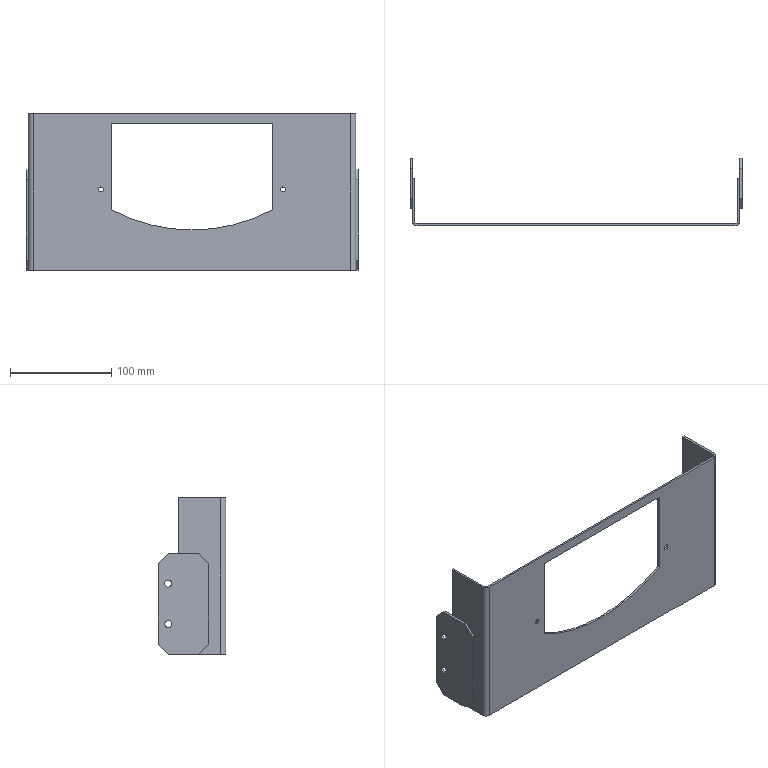Part | NX | features BREP 3 | 3 solids | 50 faces | box 328 x 67 x 155 mm | volume 114572 mm3 | plane 33 | cylinder 17 | commonest cylinder face diameters 7 x8 4.917 x4 6 x2 10 x2 340 x1
STEP:
#1=CARTESIAN_POINT('',(324.,21.928,133.322));
#2=VERTEX_POINT('',#1);
#3=CARTESIAN_POINT('',(326.,21.928,133.322));
#4=VERTEX_POINT('',#3);
#5=CARTESIAN_POINT('',(2.845,21.928,133.322));
#6=DIRECTION('',(-1.,0.,0.));
#7=VECTOR('',#6,1000.);
#8=LINE('',#5,#7);
#9=EDGE_CURVE('',#2,#4,#8,.F.);
#10=ORIENTED_EDGE('',*,*,#9,.T.);
#11=CARTESIAN_POINT('',(326.,28.072,136.678));
#12=VERTEX_POINT('',#11);
#13=CARTESIAN_POINT('',(326.,25.,135.));
#14=DIRECTION('',(-1.,0.,0.));
#15=DIRECTION('',(0.,0.,-1.));
#16=AXIS2_PLACEMENT_3D('',#13,#14,#15);
#17=CIRCLE('',#16,3.5);
#18=EDGE_CURVE('',#12,#4,#17,.T.);
#19=ORIENTED_EDGE('',*,*,#18,.F.);
#20=CARTESIAN_POINT('',(324.,28.072,136.678));
#21=VERTEX_POINT('',#20);
#22=CARTESIAN_POINT('',(2.845,28.072,136.678));
#23=DIRECTION('',(-1.,0.,0.));
#24=VECTOR('',#23,1000.);
#25=LINE('',#22,#24);
#26=EDGE_CURVE('',#21,#12,#25,.F.);
#27=ORIENTED_EDGE('',*,*,#26,.F.);
#28=CARTESIAN_POINT('',(324.,25.,135.));
#29=DIRECTION('',(-1.,0.,0.));
#30=DIRECTION('',(0.,0.,-1.));
#31=AXIS2_PLACEMENT_3D('',#28,#29,#30);
#32=CIRCLE('',#31,3.5);
#33=EDGE_CURVE('',#21,#2,#32,.T.);
#34=ORIENTED_EDGE('',*,*,#33,.T.);
#35=EDGE_LOOP('',(#10,#19,#27,#34));
#36=FACE_BOUND('',#35,.T.);
#37=CARTESIAN_POINT('',(-1.9,25.,135.));
#38=DIRECTION('',(1.,0.,0.));
#39=DIRECTION('',(0.,-0.8776,-0.4794));
#40=AXIS2_PLACEMENT_3D('',#37,#38,#39);
#41=CYLINDRICAL_SURFACE('',#40,3.5);
#42=ADVANCED_FACE('',(#36),#41,.F.);
#43=ORIENTED_EDGE('',*,*,#26,.T.);
#44=CARTESIAN_POINT('',(326.,25.,135.));
#45=DIRECTION('',(-1.,0.,0.));
#46=DIRECTION('',(0.,0.,-1.));
#47=AXIS2_PLACEMENT_3D('',#44,#45,#46);
#48=CIRCLE('',#47,3.5);
#49=EDGE_CURVE('',#4,#12,#48,.T.);
#50=ORIENTED_EDGE('',*,*,#49,.F.);
#51=ORIENTED_EDGE('',*,*,#9,.F.);
#52=CARTESIAN_POINT('',(324.,25.,135.));
#53=DIRECTION('',(-1.,0.,0.));
#54=DIRECTION('',(0.,0.,-1.));
#55=AXIS2_PLACEMENT_3D('',#52,#53,#54);
#56=CIRCLE('',#55,3.5);
#57=EDGE_CURVE('',#2,#21,#56,.T.);
#58=ORIENTED_EDGE('',*,*,#57,.T.);
#59=EDGE_LOOP('',(#43,#50,#51,#58));
#60=FACE_BOUND('',#59,.T.);
#61=CARTESIAN_POINT('',(-1.9,25.,135.));
#62=DIRECTION('',(1.,0.,0.));
#63=DIRECTION('',(0.,-0.8776,-0.4794));
#64=AXIS2_PLACEMENT_3D('',#61,#62,#63);
#65=CYLINDRICAL_SURFACE('',#64,3.5);
#66=ADVANCED_FACE('',(#60),#65,.F.);
#67=CARTESIAN_POINT('',(326.,-15.,115.));
#68=VERTEX_POINT('',#67);
#69=CARTESIAN_POINT('',(326.,-15.,195.));
#70=VERTEX_POINT('',#69);
#71=CARTESIAN_POINT('',(326.,-15.,155.));
#72=DIRECTION('',(0.,0.,1.));
#73=VECTOR('',#72,1000.);
#74=LINE('',#71,#73);
#75=EDGE_CURVE('',#68,#70,#74,.T.);
#76=ORIENTED_EDGE('',*,*,#75,.T.);
#77=CARTESIAN_POINT('',(324.,-15.,195.));
#78=VERTEX_POINT('',#77);
#79=CARTESIAN_POINT('',(325.,-15.,195.));
#80=DIRECTION('',(-1.,0.,0.));
#81=VECTOR('',#80,1000.);
#82=LINE('',#79,#81);
#83=EDGE_CURVE('',#70,#78,#82,.T.);
#84=ORIENTED_EDGE('',*,*,#83,.T.);
#85=CARTESIAN_POINT('',(324.,-15.,115.));
#86=VERTEX_POINT('',#85);
#87=CARTESIAN_POINT('',(324.,-15.,155.));
#88=DIRECTION('',(0.,0.,1.));
#89=VECTOR('',#88,1000.);
#90=LINE('',#87,#89);
#91=EDGE_CURVE('',#86,#78,#90,.T.);
#92=ORIENTED_EDGE('',*,*,#91,.F.);
#93=CARTESIAN_POINT('',(325.,-15.,115.));
#94=DIRECTION('',(-1.,0.,0.));
#95=VECTOR('',#94,1000.);
#96=LINE('',#93,#95);
#97=EDGE_CURVE('',#68,#86,#96,.T.);
#98=ORIENTED_EDGE('',*,*,#97,.F.);
#99=EDGE_LOOP('',(#76,#84,#92,#98));
#100=FACE_BOUND('',#99,.T.);
#101=CARTESIAN_POINT('',(0.,-15.,105.));
#102=DIRECTION('',(0.,-1.,0.));
#103=DIRECTION('',(0.,0.,-1.));
#104=AXIS2_PLACEMENT_3D('',#101,#102,#103);
#105=PLANE('',#104);
#106=ADVANCED_FACE('',(#100),#105,.T.);
#107=CARTESIAN_POINT('',(326.,25.,205.));
#108=VERTEX_POINT('',#107);
#109=CARTESIAN_POINT('',(324.,25.,205.));
#110=VERTEX_POINT('',#109);
#111=CARTESIAN_POINT('',(325.,25.,205.));
#112=DIRECTION('',(-1.,0.,0.));
#113=VECTOR('',#112,1000.);
#114=LINE('',#111,#113);
#115=EDGE_CURVE('',#108,#110,#114,.T.);
#116=ORIENTED_EDGE('',*,*,#115,.T.);
#117=CARTESIAN_POINT('',(324.,-5.,205.));
#118=VERTEX_POINT('',#117);
#119=CARTESIAN_POINT('',(324.,10.,205.));
#120=DIRECTION('',(0.,1.,0.));
#121=VECTOR('',#120,1000.);
#122=LINE('',#119,#121);
#123=EDGE_CURVE('',#118,#110,#122,.T.);
#124=ORIENTED_EDGE('',*,*,#123,.F.);
#125=CARTESIAN_POINT('',(326.,-5.,205.));
#126=VERTEX_POINT('',#125);
#127=CARTESIAN_POINT('',(325.,-5.,205.));
#128=DIRECTION('',(-1.,0.,0.));
#129=VECTOR('',#128,1000.);
#130=LINE('',#127,#129);
#131=EDGE_CURVE('',#126,#118,#130,.T.);
#132=ORIENTED_EDGE('',*,*,#131,.F.);
#133=CARTESIAN_POINT('',(326.,10.,205.));
#134=DIRECTION('',(0.,1.,0.));
#135=VECTOR('',#134,1000.);
#136=LINE('',#133,#135);
#137=EDGE_CURVE('',#126,#108,#136,.T.);
#138=ORIENTED_EDGE('',*,*,#137,.T.);
#139=EDGE_LOOP('',(#116,#124,#132,#138));
#140=FACE_BOUND('',#139,.T.);
#141=CARTESIAN_POINT('',(0.,35.,205.));
#142=DIRECTION('',(0.,0.,-1.));
#143=DIRECTION('',(0.,1.,0.));
#144=AXIS2_PLACEMENT_3D('',#141,#142,#143);
#145=PLANE('',#144);
#146=ADVANCED_FACE('',(#140),#145,.F.);
#147=CARTESIAN_POINT('',(324.,35.,195.));
#148=VERTEX_POINT('',#147);
#149=CARTESIAN_POINT('',(324.,35.,115.));
#150=VERTEX_POINT('',#149);
#151=CARTESIAN_POINT('',(324.,35.,155.));
#152=DIRECTION('',(0.,0.,-1.));
#153=VECTOR('',#152,1000.);
#154=LINE('',#151,#153);
#155=EDGE_CURVE('',#148,#150,#154,.T.);
#156=ORIENTED_EDGE('',*,*,#155,.F.);
#157=CARTESIAN_POINT('',(326.,35.,195.));
#158=VERTEX_POINT('',#157);
#159=CARTESIAN_POINT('',(325.,35.,195.));
#160=DIRECTION('',(-1.,0.,0.));
#161=VECTOR('',#160,1000.);
#162=LINE('',#159,#161);
#163=EDGE_CURVE('',#158,#148,#162,.T.);
#164=ORIENTED_EDGE('',*,*,#163,.F.);
#165=CARTESIAN_POINT('',(326.,35.,115.));
#166=VERTEX_POINT('',#165);
#167=CARTESIAN_POINT('',(326.,35.,155.));
#168=DIRECTION('',(0.,0.,-1.));
#169=VECTOR('',#168,1000.);
#170=LINE('',#167,#169);
#171=EDGE_CURVE('',#158,#166,#170,.T.);
#172=ORIENTED_EDGE('',*,*,#171,.T.);
#173=CARTESIAN_POINT('',(325.,35.,115.));
#174=DIRECTION('',(-1.,0.,0.));
#175=VECTOR('',#174,1000.);
#176=LINE('',#173,#175);
#177=EDGE_CURVE('',#166,#150,#176,.T.);
#178=ORIENTED_EDGE('',*,*,#177,.T.);
#179=EDGE_LOOP('',(#156,#164,#172,#178));
#180=FACE_BOUND('',#179,.T.);
#181=CARTESIAN_POINT('',(0.,35.,205.));
#182=DIRECTION('',(0.,1.,0.));
#183=DIRECTION('',(0.,0.,1.));
#184=AXIS2_PLACEMENT_3D('',#181,#182,#183);
#185=PLANE('',#184);
#186=ADVANCED_FACE('',(#180),#185,.T.);
#187=CARTESIAN_POINT('',(326.,-5.,105.));
#188=VERTEX_POINT('',#187);
#189=CARTESIAN_POINT('',(324.,-5.,105.));
#190=VERTEX_POINT('',#189);
#191=CARTESIAN_POINT('',(325.,-5.,105.));
#192=DIRECTION('',(-1.,0.,0.));
#193=VECTOR('',#192,1000.);
#194=LINE('',#191,#193);
#195=EDGE_CURVE('',#188,#190,#194,.T.);
#196=ORIENTED_EDGE('',*,*,#195,.T.);
#197=CARTESIAN_POINT('',(324.,25.,105.));
#198=VERTEX_POINT('',#197);
#199=CARTESIAN_POINT('',(324.,10.,105.));
#200=DIRECTION('',(0.,-1.,0.));
#201=VECTOR('',#200,1000.);
#202=LINE('',#199,#201);
#203=EDGE_CURVE('',#198,#190,#202,.T.);
#204=ORIENTED_EDGE('',*,*,#203,.F.);
#205=CARTESIAN_POINT('',(326.,25.,105.));
#206=VERTEX_POINT('',#205);
#207=CARTESIAN_POINT('',(325.,25.,105.));
#208=DIRECTION('',(-1.,0.,0.));
#209=VECTOR('',#208,1000.);
#210=LINE('',#207,#209);
#211=EDGE_CURVE('',#206,#198,#210,.T.);
#212=ORIENTED_EDGE('',*,*,#211,.F.);
#213=CARTESIAN_POINT('',(326.,10.,105.));
#214=DIRECTION('',(0.,-1.,0.));
#215=VECTOR('',#214,1000.);
#216=LINE('',#213,#215);
#217=EDGE_CURVE('',#206,#188,#216,.T.);
#218=ORIENTED_EDGE('',*,*,#217,.T.);
#219=EDGE_LOOP('',(#196,#204,#212,#218));
#220=FACE_BOUND('',#219,.T.);
#221=CARTESIAN_POINT('',(0.,-15.,105.));
#222=DIRECTION('',(0.,0.,1.));
#223=DIRECTION('',(0.,-1.,0.));
#224=AXIS2_PLACEMENT_3D('',#221,#222,#223);
#225=PLANE('',#224);
#226=ADVANCED_FACE('',(#220),#225,.F.);
#227=CARTESIAN_POINT('',(324.,-10.,110.));
#228=DIRECTION('',(0.,0.7071,-0.7071));
#229=VECTOR('',#228,1000.);
#230=LINE('',#227,#229);
#231=EDGE_CURVE('',#86,#190,#230,.T.);
#232=ORIENTED_EDGE('',*,*,#231,.T.);
#233=ORIENTED_EDGE('',*,*,#195,.F.);
#234=CARTESIAN_POINT('',(326.,-10.,110.));
#235=DIRECTION('',(0.,-0.7071,0.7071));
#236=VECTOR('',#235,1000.);
#237=LINE('',#234,#236);
#238=EDGE_CURVE('',#188,#68,#237,.T.);
#239=ORIENTED_EDGE('',*,*,#238,.T.);
#240=ORIENTED_EDGE('',*,*,#97,.T.);
#241=EDGE_LOOP('',(#232,#233,#239,#240));
#242=FACE_BOUND('',#241,.T.);
#243=CARTESIAN_POINT('',(-2.4,-5.,105.));
#244=DIRECTION('',(0.,-0.7071,-0.7071));
#245=DIRECTION('',(-1.,0.,0.));
#246=AXIS2_PLACEMENT_3D('',#243,#244,#245);
#247=PLANE('',#246);
#248=ADVANCED_FACE('',(#242),#247,.T.);
#249=CARTESIAN_POINT('',(324.,30.,110.));
#250=DIRECTION('',(0.,0.7071,0.7071));
#251=VECTOR('',#250,1000.);
#252=LINE('',#249,#251);
#253=EDGE_CURVE('',#198,#150,#252,.T.);
#254=ORIENTED_EDGE('',*,*,#253,.T.);
#255=ORIENTED_EDGE('',*,*,#177,.F.);
#256=CARTESIAN_POINT('',(326.,30.,110.));
#257=DIRECTION('',(0.,-0.7071,-0.7071));
#258=VECTOR('',#257,1000.);
#259=LINE('',#256,#258);
#260=EDGE_CURVE('',#166,#206,#259,.T.);
#261=ORIENTED_EDGE('',*,*,#260,.T.);
#262=ORIENTED_EDGE('',*,*,#211,.T.);
#263=EDGE_LOOP('',(#254,#255,#261,#262));
#264=FACE_BOUND('',#263,.T.);
#265=CARTESIAN_POINT('',(0.4,25.,105.));
#266=DIRECTION('',(0.,0.7071,-0.7071));
#267=DIRECTION('',(1.,0.,0.));
#268=AXIS2_PLACEMENT_3D('',#265,#266,#267);
#269=PLANE('',#268);
#270=ADVANCED_FACE('',(#264),#269,.T.);
#271=CARTESIAN_POINT('',(324.,30.,200.));
#272=DIRECTION('',(0.,-0.7071,0.7071));
#273=VECTOR('',#272,1000.);
#274=LINE('',#271,#273);
#275=EDGE_CURVE('',#148,#110,#274,.T.);
#276=ORIENTED_EDGE('',*,*,#275,.T.);
#277=ORIENTED_EDGE('',*,*,#115,.F.);
#278=CARTESIAN_POINT('',(326.,30.,200.));
#279=DIRECTION('',(0.,0.7071,-0.7071));
#280=VECTOR('',#279,1000.);
#281=LINE('',#278,#280);
#282=EDGE_CURVE('',#108,#158,#281,.T.);
#283=ORIENTED_EDGE('',*,*,#282,.T.);
#284=ORIENTED_EDGE('',*,*,#163,.T.);
#285=EDGE_LOOP('',(#276,#277,#283,#284));
#286=FACE_BOUND('',#285,.T.);
#287=CARTESIAN_POINT('',(-2.4,25.,205.));
#288=DIRECTION('',(0.,0.7071,0.7071));
#289=DIRECTION('',(-1.,0.,0.));
#290=AXIS2_PLACEMENT_3D('',#287,#288,#289);
#291=PLANE('',#290);
#292=ADVANCED_FACE('',(#286),#291,.T.);
#293=CARTESIAN_POINT('',(324.,-10.,200.));
#294=DIRECTION('',(0.,-0.7071,-0.7071));
#295=VECTOR('',#294,1000.);
#296=LINE('',#293,#295);
#297=EDGE_CURVE('',#118,#78,#296,.T.);
#298=ORIENTED_EDGE('',*,*,#297,.T.);
#299=ORIENTED_EDGE('',*,*,#83,.F.);
#300=CARTESIAN_POINT('',(326.,-10.,200.));
#301=DIRECTION('',(0.,0.7071,0.7071));
#302=VECTOR('',#301,1000.);
#303=LINE('',#300,#302);
#304=EDGE_CURVE('',#70,#126,#303,.T.);
#305=ORIENTED_EDGE('',*,*,#304,.T.);
#306=ORIENTED_EDGE('',*,*,#131,.T.);
#307=EDGE_LOOP('',(#298,#299,#305,#306));
#308=FACE_BOUND('',#307,.T.);
#309=CARTESIAN_POINT('',(0.4,-5.,205.));
#310=DIRECTION('',(0.,-0.7071,0.7071));
#311=DIRECTION('',(1.,0.,0.));
#312=AXIS2_PLACEMENT_3D('',#309,#310,#311);
#313=PLANE('',#312);
#314=ADVANCED_FACE('',(#308),#313,.T.);
#315=ORIENTED_EDGE('',*,*,#238,.F.);
#316=ORIENTED_EDGE('',*,*,#217,.F.);
#317=ORIENTED_EDGE('',*,*,#260,.F.);
#318=ORIENTED_EDGE('',*,*,#171,.F.);
#319=ORIENTED_EDGE('',*,*,#282,.F.);
#320=ORIENTED_EDGE('',*,*,#137,.F.);
#321=ORIENTED_EDGE('',*,*,#304,.F.);
#322=ORIENTED_EDGE('',*,*,#75,.F.);
#323=EDGE_LOOP('',(#315,#316,#317,#318,#319,#320,#321,#322));
#324=FACE_BOUND('',#323,.T.);
#325=CARTESIAN_POINT('',(326.,21.928,173.322));
#326=VERTEX_POINT('',#325);
#327=CARTESIAN_POINT('',(326.,28.072,176.678));
#328=VERTEX_POINT('',#327);
#329=CARTESIAN_POINT('',(326.,25.,175.));
#330=DIRECTION('',(-1.,0.,0.));
#331=DIRECTION('',(0.,0.,1.));
#332=AXIS2_PLACEMENT_3D('',#329,#330,#331);
#333=CIRCLE('',#332,3.5);
#334=EDGE_CURVE('',#326,#328,#333,.T.);
#335=ORIENTED_EDGE('',*,*,#334,.T.);
#336=CARTESIAN_POINT('',(326.,25.,175.));
#337=DIRECTION('',(-1.,0.,0.));
#338=DIRECTION('',(0.,0.,1.));
#339=AXIS2_PLACEMENT_3D('',#336,#337,#338);
#340=CIRCLE('',#339,3.5);
#341=EDGE_CURVE('',#328,#326,#340,.T.);
#342=ORIENTED_EDGE('',*,*,#341,.T.);
#343=EDGE_LOOP('',(#335,#342));
#344=FACE_BOUND('',#343,.T.);
#345=ORIENTED_EDGE('',*,*,#18,.T.);
#346=ORIENTED_EDGE('',*,*,#49,.T.);
#347=EDGE_LOOP('',(#345,#346));
#348=FACE_BOUND('',#347,.T.);
#349=CARTESIAN_POINT('',(326.,0.,0.));
#350=DIRECTION('',(-1.,0.,0.));
#351=DIRECTION('',(0.,1.,0.));
#352=AXIS2_PLACEMENT_3D('',#349,#350,#351);
#353=PLANE('',#352);
#354=ADVANCED_FACE('',(#324,#344,#348),#353,.F.);
#355=ORIENTED_EDGE('',*,*,#91,.T.);
#356=ORIENTED_EDGE('',*,*,#297,.F.);
#357=ORIENTED_EDGE('',*,*,#123,.T.);
#358=ORIENTED_EDGE('',*,*,#275,.F.);
#359=ORIENTED_EDGE('',*,*,#155,.T.);
#360=ORIENTED_EDGE('',*,*,#253,.F.);
#361=ORIENTED_EDGE('',*,*,#203,.T.);
#362=ORIENTED_EDGE('',*,*,#231,.F.);
#363=EDGE_LOOP('',(#355,#356,#357,#358,#359,#360,#361,#362));
#364=FACE_BOUND('',#363,.T.);
#365=CARTESIAN_POINT('',(324.,28.072,176.678));
#366=VERTEX_POINT('',#365);
#367=CARTESIAN_POINT('',(324.,21.928,173.322));
#368=VERTEX_POINT('',#367);
#369=CARTESIAN_POINT('',(324.,25.,175.));
#370=DIRECTION('',(-1.,0.,0.));
#371=DIRECTION('',(0.,0.,1.));
#372=AXIS2_PLACEMENT_3D('',#369,#370,#371);
#373=CIRCLE('',#372,3.5);
#374=EDGE_CURVE('',#366,#368,#373,.T.);
#375=ORIENTED_EDGE('',*,*,#374,.F.);
#376=CARTESIAN_POINT('',(324.,25.,175.));
#377=DIRECTION('',(-1.,0.,0.));
#378=DIRECTION('',(0.,0.,1.));
#379=AXIS2_PLACEMENT_3D('',#376,#377,#378);
#380=CIRCLE('',#379,3.5);
#381=EDGE_CURVE('',#368,#366,#380,.T.);
#382=ORIENTED_EDGE('',*,*,#381,.F.);
#383=EDGE_LOOP('',(#375,#382));
#384=FACE_BOUND('',#383,.T.);
#385=ORIENTED_EDGE('',*,*,#57,.F.);
#386=ORIENTED_EDGE('',*,*,#33,.F.);
#387=EDGE_LOOP('',(#385,#386));
#388=FACE_BOUND('',#387,.T.);
#389=CARTESIAN_POINT('',(324.,0.,0.));
#390=DIRECTION('',(-1.,0.,0.));
#391=DIRECTION('',(0.,1.,0.));
#392=AXIS2_PLACEMENT_3D('',#389,#390,#391);
#393=PLANE('',#392);
#394=ADVANCED_FACE('',(#364,#384,#388),#393,.T.);
#395=CARTESIAN_POINT('',(2.845,21.928,173.322));
#396=DIRECTION('',(-1.,0.,0.));
#397=VECTOR('',#396,1000.);
#398=LINE('',#395,#397);
#399=EDGE_CURVE('',#368,#326,#398,.F.);
#400=ORIENTED_EDGE('',*,*,#399,.T.);
#401=ORIENTED_EDGE('',*,*,#341,.F.);
#402=CARTESIAN_POINT('',(2.845,28.072,176.678));
#403=DIRECTION('',(-1.,0.,0.));
#404=VECTOR('',#403,1000.);
#405=LINE('',#402,#404);
#406=EDGE_CURVE('',#366,#328,#405,.F.);
#407=ORIENTED_EDGE('',*,*,#406,.F.);
#408=ORIENTED_EDGE('',*,*,#374,.T.);
#409=EDGE_LOOP('',(#400,#401,#407,#408));
#410=FACE_BOUND('',#409,.T.);
#411=CARTESIAN_POINT('',(-1.9,25.,175.));
#412=DIRECTION('',(1.,0.,0.));
#413=DIRECTION('',(0.,-0.8776,-0.4794));
#414=AXIS2_PLACEMENT_3D('',#411,#412,#413);
#415=CYLINDRICAL_SURFACE('',#414,3.5);
#416=ADVANCED_FACE('',(#410),#415,.F.);
#417=ORIENTED_EDGE('',*,*,#406,.T.);
#418=ORIENTED_EDGE('',*,*,#334,.F.);
#419=ORIENTED_EDGE('',*,*,#399,.F.);
#420=ORIENTED_EDGE('',*,*,#381,.T.);
#421=EDGE_LOOP('',(#417,#418,#419,#420));
#422=FACE_BOUND('',#421,.T.);
#423=CARTESIAN_POINT('',(-1.9,25.,175.));
#424=DIRECTION('',(1.,0.,0.));
#425=DIRECTION('',(0.,-0.8776,-0.4794));
#426=AXIS2_PLACEMENT_3D('',#423,#424,#425);
#427=CYLINDRICAL_SURFACE('',#426,3.5);
#428=ADVANCED_FACE('',(#422),#427,.F.);
#429=CLOSED_SHELL('',(#42,#66,#106,#146,#186,#226,#248,#270,#292,#314,#354,#394,#416,#428));
#430=MANIFOLD_SOLID_BREP('',#429);
#431=CARTESIAN_POINT('',(69.842,-32.,186.179));
#432=VERTEX_POINT('',#431);
#433=CARTESIAN_POINT('',(69.842,-30.,186.179));
#434=VERTEX_POINT('',#433);
#435=CARTESIAN_POINT('',(69.842,-27.155,186.179));
#436=DIRECTION('',(0.,-1.,0.));
#437=VECTOR('',#436,1000.);
#438=LINE('',#435,#437);
#439=EDGE_CURVE('',#432,#434,#438,.F.);
#440=ORIENTED_EDGE('',*,*,#439,.T.);
#441=CARTESIAN_POINT('',(74.157,-30.,183.821));
#442=VERTEX_POINT('',#441);
#443=CARTESIAN_POINT('',(72.,-30.,185.));
#444=DIRECTION('',(0.,-1.,0.));
#445=DIRECTION('',(1.,0.,0.));
#446=AXIS2_PLACEMENT_3D('',#443,#444,#445);
#447=CIRCLE('',#446,2.458);
#448=EDGE_CURVE('',#442,#434,#447,.T.);
#449=ORIENTED_EDGE('',*,*,#448,.F.);
#450=CARTESIAN_POINT('',(74.157,-32.,183.821));
#451=VERTEX_POINT('',#450);
#452=CARTESIAN_POINT('',(74.157,-27.155,183.821));
#453=DIRECTION('',(0.,-1.,0.));
#454=VECTOR('',#453,1000.);
#455=LINE('',#452,#454);
#456=EDGE_CURVE('',#451,#442,#455,.F.);
#457=ORIENTED_EDGE('',*,*,#456,.F.);
#458=CARTESIAN_POINT('',(72.,-32.,185.));
#459=DIRECTION('',(0.,-1.,0.));
#460=DIRECTION('',(1.,0.,0.));
#461=AXIS2_PLACEMENT_3D('',#458,#459,#460);
#462=CIRCLE('',#461,2.458);
#463=EDGE_CURVE('',#451,#432,#462,.T.);
#464=ORIENTED_EDGE('',*,*,#463,.T.);
#465=EDGE_LOOP('',(#440,#449,#457,#464));
#466=FACE_BOUND('',#465,.T.);
#467=CARTESIAN_POINT('',(72.,-31.9,185.));
#468=DIRECTION('',(0.,1.,0.));
#469=DIRECTION('',(-0.8776,0.,0.4794));
#470=AXIS2_PLACEMENT_3D('',#467,#468,#469);
#471=CYLINDRICAL_SURFACE('',#470,2.458);
#472=ADVANCED_FACE('',(#466),#471,.F.);
#473=ORIENTED_EDGE('',*,*,#456,.T.);
#474=CARTESIAN_POINT('',(72.,-30.,185.));
#475=DIRECTION('',(0.,-1.,0.));
#476=DIRECTION('',(1.,0.,0.));
#477=AXIS2_PLACEMENT_3D('',#474,#475,#476);
#478=CIRCLE('',#477,2.458);
#479=EDGE_CURVE('',#434,#442,#478,.T.);
#480=ORIENTED_EDGE('',*,*,#479,.F.);
#481=ORIENTED_EDGE('',*,*,#439,.F.);
#482=CARTESIAN_POINT('',(72.,-32.,185.));
#483=DIRECTION('',(0.,-1.,0.));
#484=DIRECTION('',(1.,0.,0.));
#485=AXIS2_PLACEMENT_3D('',#482,#483,#484);
#486=CIRCLE('',#485,2.458);
#487=EDGE_CURVE('',#432,#451,#486,.T.);
#488=ORIENTED_EDGE('',*,*,#487,.T.);
#489=EDGE_LOOP('',(#473,#480,#481,#488));
#490=FACE_BOUND('',#489,.T.);
#491=CARTESIAN_POINT('',(72.,-31.9,185.));
#492=DIRECTION('',(0.,1.,0.));
#493=DIRECTION('',(-0.8776,0.,0.4794));
#494=AXIS2_PLACEMENT_3D('',#491,#492,#493);
#495=CYLINDRICAL_SURFACE('',#494,2.458);
#496=ADVANCED_FACE('',(#490),#495,.F.);
#497=CARTESIAN_POINT('',(2.,15.,260.));
#498=VERTEX_POINT('',#497);
#499=CARTESIAN_POINT('',(2.,15.,105.));
#500=VERTEX_POINT('',#499);
#501=CARTESIAN_POINT('',(2.,15.,182.5));
#502=DIRECTION('',(0.,0.,-1.));
#503=VECTOR('',#502,1000.);
#504=LINE('',#501,#503);
#505=EDGE_CURVE('',#498,#500,#504,.T.);
#506=ORIENTED_EDGE('',*,*,#505,.T.);
#507=CARTESIAN_POINT('',(0.,15.,105.));
#508=VERTEX_POINT('',#507);
#509=CARTESIAN_POINT('',(1.,15.,105.));
#510=DIRECTION('',(-1.,0.,0.));
#511=VECTOR('',#510,1000.);
#512=LINE('',#509,#511);
#513=EDGE_CURVE('',#500,#508,#512,.T.);
#514=ORIENTED_EDGE('',*,*,#513,.T.);
#515=CARTESIAN_POINT('',(0.,15.,260.));
#516=VERTEX_POINT('',#515);
#517=CARTESIAN_POINT('',(0.,15.,182.5));
#518=DIRECTION('',(0.,0.,-1.));
#519=VECTOR('',#518,1000.);
#520=LINE('',#517,#519);
#521=EDGE_CURVE('',#516,#508,#520,.T.);
#522=ORIENTED_EDGE('',*,*,#521,.F.);
#523=CARTESIAN_POINT('',(1.,15.,260.));
#524=DIRECTION('',(1.,0.,0.));
#525=VECTOR('',#524,1000.);
#526=LINE('',#523,#525);
#527=EDGE_CURVE('',#516,#498,#526,.T.);
#528=ORIENTED_EDGE('',*,*,#527,.T.);
#529=EDGE_LOOP('',(#506,#514,#522,#528));
#530=FACE_BOUND('',#529,.T.);
#531=CARTESIAN_POINT('',(324.,15.,20.));
#532=DIRECTION('',(0.,-1.,0.));
#533=DIRECTION('',(0.,0.,1.));
#534=AXIS2_PLACEMENT_3D('',#531,#532,#533);
#535=PLANE('',#534);
#536=ADVANCED_FACE('',(#530),#535,.F.);
#537=CARTESIAN_POINT('',(322.,15.,105.));
#538=VERTEX_POINT('',#537);
#539=CARTESIAN_POINT('',(322.,15.,260.));
#540=VERTEX_POINT('',#539);
#541=CARTESIAN_POINT('',(322.,15.,182.5));
#542=DIRECTION('',(0.,0.,1.));
#543=VECTOR('',#542,1000.);
#544=LINE('',#541,#543);
#545=EDGE_CURVE('',#538,#540,#544,.T.);
#546=ORIENTED_EDGE('',*,*,#545,.T.);
#547=CARTESIAN_POINT('',(324.,15.,260.));
#548=VERTEX_POINT('',#547);
#549=CARTESIAN_POINT('',(323.,15.,260.));
#550=DIRECTION('',(1.,0.,0.));
#551=VECTOR('',#550,1000.);
#552=LINE('',#549,#551);
#553=EDGE_CURVE('',#540,#548,#552,.T.);
#554=ORIENTED_EDGE('',*,*,#553,.T.);
#555=CARTESIAN_POINT('',(324.,15.,105.));
#556=VERTEX_POINT('',#555);
#557=CARTESIAN_POINT('',(324.,15.,182.5));
#558=DIRECTION('',(0.,0.,1.));
#559=VECTOR('',#558,1000.);
#560=LINE('',#557,#559);
#561=EDGE_CURVE('',#556,#548,#560,.T.);
#562=ORIENTED_EDGE('',*,*,#561,.F.);
#563=CARTESIAN_POINT('',(323.,15.,105.));
#564=DIRECTION('',(-1.,0.,0.));
#565=VECTOR('',#564,1000.);
#566=LINE('',#563,#565);
#567=EDGE_CURVE('',#556,#538,#566,.T.);
#568=ORIENTED_EDGE('',*,*,#567,.T.);
#569=EDGE_LOOP('',(#546,#554,#562,#568));
#570=FACE_BOUND('',#569,.T.);
#571=CARTESIAN_POINT('',(324.,15.,20.));
#572=DIRECTION('',(0.,-1.,0.));
#573=DIRECTION('',(0.,0.,1.));
#574=AXIS2_PLACEMENT_3D('',#571,#572,#573);
#575=PLANE('',#574);
#576=ADVANCED_FACE('',(#570),#575,.F.);
#577=CARTESIAN_POINT('',(82.,-30.,250.));
#578=VERTEX_POINT('',#577);
#579=CARTESIAN_POINT('',(242.,-30.,250.));
#580=VERTEX_POINT('',#579);
#581=CARTESIAN_POINT('',(162.,-30.,250.));
#582=DIRECTION('',(1.,0.,0.));
#583=VECTOR('',#582,1000.);
#584=LINE('',#581,#583);
#585=EDGE_CURVE('',#578,#580,#584,.T.);
#586=ORIENTED_EDGE('',*,*,#585,.T.);
#587=CARTESIAN_POINT('',(242.,-32.,250.));
#588=VERTEX_POINT('',#587);
#589=CARTESIAN_POINT('',(242.,-31.,250.));
#590=DIRECTION('',(0.,1.,0.));
#591=VECTOR('',#590,1000.);
#592=LINE('',#589,#591);
#593=EDGE_CURVE('',#588,#580,#592,.T.);
#594=ORIENTED_EDGE('',*,*,#593,.F.);
#595=CARTESIAN_POINT('',(82.,-32.,250.));
#596=VERTEX_POINT('',#595);
#597=CARTESIAN_POINT('',(162.,-32.,250.));
#598=DIRECTION('',(-1.,0.,0.));
#599=VECTOR('',#598,1000.);
#600=LINE('',#597,#599);
#601=EDGE_CURVE('',#588,#596,#600,.T.);
#602=ORIENTED_EDGE('',*,*,#601,.T.);
#603=CARTESIAN_POINT('',(82.,-31.,250.));
#604=DIRECTION('',(0.,1.,0.));
#605=VECTOR('',#604,1000.);
#606=LINE('',#603,#605);
#607=EDGE_CURVE('',#596,#578,#606,.T.);
#608=ORIENTED_EDGE('',*,*,#607,.T.);
#609=EDGE_LOOP('',(#586,#594,#602,#608));
#610=FACE_BOUND('',#609,.T.);
#611=CARTESIAN_POINT('',(82.,-32.,250.));
#612=DIRECTION('',(0.,0.,1.));
#613=DIRECTION('',(-1.,0.,0.));
#614=AXIS2_PLACEMENT_3D('',#611,#612,#613);
#615=PLANE('',#614);
#616=ADVANCED_FACE('',(#610),#615,.F.);
#617=ORIENTED_EDGE('',*,*,#607,.F.);
#618=CARTESIAN_POINT('',(82.,-32.,165.));
#619=VERTEX_POINT('',#618);
#620=CARTESIAN_POINT('',(82.,-32.,207.5));
#621=DIRECTION('',(0.,0.,-1.));
#622=VECTOR('',#621,1000.);
#623=LINE('',#620,#622);
#624=EDGE_CURVE('',#596,#619,#623,.T.);
#625=ORIENTED_EDGE('',*,*,#624,.T.);
#626=CARTESIAN_POINT('',(82.,-30.,165.));
#627=VERTEX_POINT('',#626);
#628=CARTESIAN_POINT('',(82.,-31.,165.));
#629=DIRECTION('',(0.,1.,0.));
#630=VECTOR('',#629,1000.);
#631=LINE('',#628,#630);
#632=EDGE_CURVE('',#619,#627,#631,.T.);
#633=ORIENTED_EDGE('',*,*,#632,.T.);
#634=CARTESIAN_POINT('',(82.,-30.,207.5));
#635=DIRECTION('',(0.,0.,-1.));
#636=VECTOR('',#635,1000.);
#637=LINE('',#634,#636);
#638=EDGE_CURVE('',#578,#627,#637,.T.);
#639=ORIENTED_EDGE('',*,*,#638,.F.);
#640=EDGE_LOOP('',(#617,#625,#633,#639));
#641=FACE_BOUND('',#640,.T.);
#642=CARTESIAN_POINT('',(82.,-32.,250.));
#643=DIRECTION('',(1.,0.,0.));
#644=DIRECTION('',(0.,0.,1.));
#645=AXIS2_PLACEMENT_3D('',#642,#643,#644);
#646=PLANE('',#645);
#647=ADVANCED_FACE('',(#641),#646,.T.);
#648=CARTESIAN_POINT('',(242.,-30.,165.));
#649=VERTEX_POINT('',#648);
#650=CARTESIAN_POINT('',(162.,-30.,315.));
#651=DIRECTION('',(0.,-1.,0.));
#652=DIRECTION('',(1.,0.,0.));
#653=AXIS2_PLACEMENT_3D('',#650,#651,#652);
#654=CIRCLE('',#653,170.);
#655=EDGE_CURVE('',#627,#649,#654,.T.);
#656=ORIENTED_EDGE('',*,*,#655,.F.);
#657=ORIENTED_EDGE('',*,*,#632,.F.);
#658=CARTESIAN_POINT('',(242.,-32.,165.));
#659=VERTEX_POINT('',#658);
#660=CARTESIAN_POINT('',(162.,-32.,315.));
#661=DIRECTION('',(0.,-1.,0.));
#662=DIRECTION('',(1.,0.,0.));
#663=AXIS2_PLACEMENT_3D('',#660,#661,#662);
#664=CIRCLE('',#663,170.);
#665=EDGE_CURVE('',#619,#659,#664,.T.);
#666=ORIENTED_EDGE('',*,*,#665,.T.);
#667=CARTESIAN_POINT('',(242.,-22.,165.));
#668=DIRECTION('',(0.,1.,0.));
#669=VECTOR('',#668,1000.);
#670=LINE('',#667,#669);
#671=EDGE_CURVE('',#659,#649,#670,.T.);
#672=ORIENTED_EDGE('',*,*,#671,.T.);
#673=EDGE_LOOP('',(#656,#657,#666,#672));
#674=FACE_BOUND('',#673,.T.);
#675=CARTESIAN_POINT('',(162.,-22.,315.));
#676=DIRECTION('',(0.,-1.,0.));
#677=DIRECTION('',(0.4706,0.,0.8824));
#678=AXIS2_PLACEMENT_3D('',#675,#676,#677);
#679=CYLINDRICAL_SURFACE('',#678,170.);
#680=ADVANCED_FACE('',(#674),#679,.F.);
#681=ORIENTED_EDGE('',*,*,#671,.F.);
#682=CARTESIAN_POINT('',(242.,-32.,207.5));
#683=DIRECTION('',(0.,0.,1.));
#684=VECTOR('',#683,1000.);
#685=LINE('',#682,#684);
#686=EDGE_CURVE('',#659,#588,#685,.T.);
#687=ORIENTED_EDGE('',*,*,#686,.T.);
#688=ORIENTED_EDGE('',*,*,#593,.T.);
#689=CARTESIAN_POINT('',(242.,-30.,207.5));
#690=DIRECTION('',(0.,0.,1.));
#691=VECTOR('',#690,1000.);
#692=LINE('',#689,#691);
#693=EDGE_CURVE('',#649,#580,#692,.T.);
#694=ORIENTED_EDGE('',*,*,#693,.F.);
#695=EDGE_LOOP('',(#681,#687,#688,#694));
#696=FACE_BOUND('',#695,.T.);
#697=CARTESIAN_POINT('',(242.,-32.,165.));
#698=DIRECTION('',(-1.,0.,0.));
#699=DIRECTION('',(0.,0.,-1.));
#700=AXIS2_PLACEMENT_3D('',#697,#698,#699);
#701=PLANE('',#700);
#702=ADVANCED_FACE('',(#696),#701,.T.);
#703=CARTESIAN_POINT('',(249.842,-32.,186.179));
#704=VERTEX_POINT('',#703);
#705=CARTESIAN_POINT('',(249.842,-30.,186.179));
#706=VERTEX_POINT('',#705);
#707=CARTESIAN_POINT('',(249.842,-27.155,186.179));
#708=DIRECTION('',(0.,-1.,0.));
#709=VECTOR('',#708,1000.);
#710=LINE('',#707,#709);
#711=EDGE_CURVE('',#704,#706,#710,.F.);
#712=ORIENTED_EDGE('',*,*,#711,.T.);
#713=CARTESIAN_POINT('',(254.157,-30.,183.821));
#714=VERTEX_POINT('',#713);
#715=CARTESIAN_POINT('',(252.,-30.,185.));
#716=DIRECTION('',(0.,-1.,0.));
#717=DIRECTION('',(1.,0.,0.));
#718=AXIS2_PLACEMENT_3D('',#715,#716,#717);
#719=CIRCLE('',#718,2.458);
#720=EDGE_CURVE('',#714,#706,#719,.T.);
#721=ORIENTED_EDGE('',*,*,#720,.F.);
#722=CARTESIAN_POINT('',(254.157,-32.,183.821));
#723=VERTEX_POINT('',#722);
#724=CARTESIAN_POINT('',(254.157,-27.155,183.821));
#725=DIRECTION('',(0.,-1.,0.));
#726=VECTOR('',#725,1000.);
#727=LINE('',#724,#726);
#728=EDGE_CURVE('',#723,#714,#727,.F.);
#729=ORIENTED_EDGE('',*,*,#728,.F.);
#730=CARTESIAN_POINT('',(252.,-32.,185.));
#731=DIRECTION('',(0.,-1.,0.));
#732=DIRECTION('',(1.,0.,0.));
#733=AXIS2_PLACEMENT_3D('',#730,#731,#732);
#734=CIRCLE('',#733,2.458);
#735=EDGE_CURVE('',#723,#704,#734,.T.);
#736=ORIENTED_EDGE('',*,*,#735,.T.);
#737=EDGE_LOOP('',(#712,#721,#729,#736));
#738=FACE_BOUND('',#737,.T.);
#739=CARTESIAN_POINT('',(252.,-31.9,185.));
#740=DIRECTION('',(0.,1.,0.));
#741=DIRECTION('',(-0.8776,0.,0.4794));
#742=AXIS2_PLACEMENT_3D('',#739,#740,#741);
#743=CYLINDRICAL_SURFACE('',#742,2.458);
#744=ADVANCED_FACE('',(#738),#743,.F.);
#745=ORIENTED_EDGE('',*,*,#728,.T.);
#746=CARTESIAN_POINT('',(252.,-30.,185.));
#747=DIRECTION('',(0.,-1.,0.));
#748=DIRECTION('',(1.,0.,0.));
#749=AXIS2_PLACEMENT_3D('',#746,#747,#748);
#750=CIRCLE('',#749,2.458);
#751=EDGE_CURVE('',#706,#714,#750,.T.);
#752=ORIENTED_EDGE('',*,*,#751,.F.);
#753=ORIENTED_EDGE('',*,*,#711,.F.);
#754=CARTESIAN_POINT('',(252.,-32.,185.));
#755=DIRECTION('',(0.,-1.,0.));
#756=DIRECTION('',(1.,0.,0.));
#757=AXIS2_PLACEMENT_3D('',#754,#755,#756);
#758=CIRCLE('',#757,2.458);
#759=EDGE_CURVE('',#704,#723,#758,.T.);
#760=ORIENTED_EDGE('',*,*,#759,.T.);
#761=EDGE_LOOP('',(#745,#752,#753,#760));
#762=FACE_BOUND('',#761,.T.);
#763=CARTESIAN_POINT('',(252.,-31.9,185.));
#764=DIRECTION('',(0.,1.,0.));
#765=DIRECTION('',(-0.8776,0.,0.4794));
#766=AXIS2_PLACEMENT_3D('',#763,#764,#765);
#767=CYLINDRICAL_SURFACE('',#766,2.458);
#768=ADVANCED_FACE('',(#762),#767,.F.);
#769=CARTESIAN_POINT('',(2.,-27.,105.));
#770=VERTEX_POINT('',#769);
#771=CARTESIAN_POINT('',(2.,-7.5,105.));
#772=DIRECTION('',(0.,1.,0.));
#773=VECTOR('',#772,1000.);
#774=LINE('',#771,#773);
#775=EDGE_CURVE('',#770,#500,#774,.T.);
#776=ORIENTED_EDGE('',*,*,#775,.T.);
#777=ORIENTED_EDGE('',*,*,#505,.F.);
#778=CARTESIAN_POINT('',(2.,-27.,260.));
#779=VERTEX_POINT('',#778);
#780=CARTESIAN_POINT('',(2.,-7.5,260.));
#781=DIRECTION('',(0.,1.,0.));
#782=VECTOR('',#781,1000.);
#783=LINE('',#780,#782);
#784=EDGE_CURVE('',#779,#498,#783,.T.);
#785=ORIENTED_EDGE('',*,*,#784,.F.);
#786=CARTESIAN_POINT('',(2.,-27.,182.5));
#787=DIRECTION('',(0.,0.,1.));
#788=VECTOR('',#787,1000.);
#789=LINE('',#786,#788);
#790=EDGE_CURVE('',#770,#779,#789,.T.);
#791=ORIENTED_EDGE('',*,*,#790,.F.);
#792=EDGE_LOOP('',(#776,#777,#785,#791));
#793=FACE_BOUND('',#792,.T.);
#794=CARTESIAN_POINT('',(2.,-32.,260.));
#795=DIRECTION('',(1.,0.,0.));
#796=DIRECTION('',(0.,0.,1.));
#797=AXIS2_PLACEMENT_3D('',#794,#795,#796);
#798=PLANE('',#797);
#799=ADVANCED_FACE('',(#793),#798,.T.);
#800=CARTESIAN_POINT('',(5.,-30.,105.));
#801=VERTEX_POINT('',#800);
#802=CARTESIAN_POINT('',(5.,-30.,260.));
#803=VERTEX_POINT('',#802);
#804=CARTESIAN_POINT('',(5.,-30.,182.5));
#805=DIRECTION('',(0.,0.,1.));
#806=VECTOR('',#805,1000.);
#807=LINE('',#804,#806);
#808=EDGE_CURVE('',#801,#803,#807,.T.);
#809=ORIENTED_EDGE('',*,*,#808,.F.);
#810=CARTESIAN_POINT('',(5.,-27.,105.));
#811=DIRECTION('',(0.,0.,1.));
#812=DIRECTION('',(-1.,0.,0.));
#813=AXIS2_PLACEMENT_3D('',#810,#811,#812);
#814=CIRCLE('',#813,3.);
#815=EDGE_CURVE('',#770,#801,#814,.T.);
#816=ORIENTED_EDGE('',*,*,#815,.F.);
#817=ORIENTED_EDGE('',*,*,#790,.T.);
#818=CARTESIAN_POINT('',(5.,-27.,260.));
#819=DIRECTION('',(0.,0.,-1.));
#820=DIRECTION('',(-1.,0.,0.));
#821=AXIS2_PLACEMENT_3D('',#818,#819,#820);
#822=CIRCLE('',#821,3.);
#823=EDGE_CURVE('',#803,#779,#822,.T.);
#824=ORIENTED_EDGE('',*,*,#823,.F.);
#825=EDGE_LOOP('',(#809,#816,#817,#824));
#826=FACE_BOUND('',#825,.T.);
#827=CARTESIAN_POINT('',(5.,-27.,182.5));
#828=DIRECTION('',(0.,0.,-1.));
#829=DIRECTION('',(0.,1.,0.));
#830=AXIS2_PLACEMENT_3D('',#827,#828,#829);
#831=CYLINDRICAL_SURFACE('',#830,3.);
#832=ADVANCED_FACE('',(#826),#831,.F.);
#833=CARTESIAN_POINT('',(322.,-27.,260.));
#834=VERTEX_POINT('',#833);
#835=CARTESIAN_POINT('',(322.,-7.5,260.));
#836=DIRECTION('',(0.,1.,0.));
#837=VECTOR('',#836,1000.);
#838=LINE('',#835,#837);
#839=EDGE_CURVE('',#834,#540,#838,.T.);
#840=ORIENTED_EDGE('',*,*,#839,.T.);
#841=ORIENTED_EDGE('',*,*,#545,.F.);
#842=CARTESIAN_POINT('',(322.,-27.,105.));
#843=VERTEX_POINT('',#842);
#844=CARTESIAN_POINT('',(322.,-7.5,105.));
#845=DIRECTION('',(0.,1.,0.));
#846=VECTOR('',#845,1000.);
#847=LINE('',#844,#846);
#848=EDGE_CURVE('',#843,#538,#847,.T.);
#849=ORIENTED_EDGE('',*,*,#848,.F.);
#850=CARTESIAN_POINT('',(322.,-27.,182.5));
#851=DIRECTION('',(0.,0.,-1.));
#852=VECTOR('',#851,1000.);
#853=LINE('',#850,#852);
#854=EDGE_CURVE('',#834,#843,#853,.T.);
#855=ORIENTED_EDGE('',*,*,#854,.F.);
#856=EDGE_LOOP('',(#840,#841,#849,#855));
#857=FACE_BOUND('',#856,.T.);
#858=CARTESIAN_POINT('',(322.,-32.,105.));
#859=DIRECTION('',(-1.,0.,0.));
#860=DIRECTION('',(0.,0.,-1.));
#861=AXIS2_PLACEMENT_3D('',#858,#859,#860);
#862=PLANE('',#861);
#863=ADVANCED_FACE('',(#857),#862,.T.);
#864=CARTESIAN_POINT('',(319.,-30.,260.));
#865=VERTEX_POINT('',#864);
#866=CARTESIAN_POINT('',(319.,-30.,105.));
#867=VERTEX_POINT('',#866);
#868=CARTESIAN_POINT('',(319.,-30.,182.5));
#869=DIRECTION('',(0.,0.,-1.));
#870=VECTOR('',#869,1000.);
#871=LINE('',#868,#870);
#872=EDGE_CURVE('',#865,#867,#871,.T.);
#873=ORIENTED_EDGE('',*,*,#872,.T.);
#874=CARTESIAN_POINT('',(162.,-30.,105.));
#875=DIRECTION('',(1.,0.,0.));
#876=VECTOR('',#875,1000.);
#877=LINE('',#874,#876);
#878=EDGE_CURVE('',#801,#867,#877,.T.);
#879=ORIENTED_EDGE('',*,*,#878,.F.);
#880=ORIENTED_EDGE('',*,*,#808,.T.);
#881=CARTESIAN_POINT('',(162.,-30.,260.));
#882=DIRECTION('',(1.,0.,0.));
#883=VECTOR('',#882,1000.);
#884=LINE('',#881,#883);
#885=EDGE_CURVE('',#803,#865,#884,.T.);
#886=ORIENTED_EDGE('',*,*,#885,.T.);
#887=EDGE_LOOP('',(#873,#879,#880,#886));
#888=FACE_BOUND('',#887,.T.);
#889=ORIENTED_EDGE('',*,*,#751,.T.);
#890=ORIENTED_EDGE('',*,*,#720,.T.);
#891=EDGE_LOOP('',(#889,#890));
#892=FACE_BOUND('',#891,.T.);
#893=ORIENTED_EDGE('',*,*,#448,.T.);
#894=ORIENTED_EDGE('',*,*,#479,.T.);
#895=EDGE_LOOP('',(#893,#894));
#896=FACE_BOUND('',#895,.T.);
#897=ORIENTED_EDGE('',*,*,#585,.F.);
#898=ORIENTED_EDGE('',*,*,#638,.T.);
#899=ORIENTED_EDGE('',*,*,#655,.T.);
#900=ORIENTED_EDGE('',*,*,#693,.T.);
#901=EDGE_LOOP('',(#897,#898,#899,#900));
#902=FACE_BOUND('',#901,.T.);
#903=CARTESIAN_POINT('',(0.,-30.,0.));
#904=DIRECTION('',(0.,-1.,0.));
#905=DIRECTION('',(-1.,0.,0.));
#906=AXIS2_PLACEMENT_3D('',#903,#904,#905);
#907=PLANE('',#906);
#908=ADVANCED_FACE('',(#888,#892,#896,#902),#907,.F.);
#909=ORIENTED_EDGE('',*,*,#872,.F.);
#910=CARTESIAN_POINT('',(319.,-27.,260.));
#911=DIRECTION('',(0.,0.,-1.));
#912=DIRECTION('',(1.,0.,0.));
#913=AXIS2_PLACEMENT_3D('',#910,#911,#912);
#914=CIRCLE('',#913,3.);
#915=EDGE_CURVE('',#834,#865,#914,.T.);
#916=ORIENTED_EDGE('',*,*,#915,.F.);
#917=ORIENTED_EDGE('',*,*,#854,.T.);
#918=CARTESIAN_POINT('',(319.,-27.,105.));
#919=DIRECTION('',(0.,0.,1.));
#920=DIRECTION('',(1.,0.,0.));
#921=AXIS2_PLACEMENT_3D('',#918,#919,#920);
#922=CIRCLE('',#921,3.);
#923=EDGE_CURVE('',#867,#843,#922,.T.);
#924=ORIENTED_EDGE('',*,*,#923,.F.);
#925=EDGE_LOOP('',(#909,#916,#917,#924));
#926=FACE_BOUND('',#925,.T.);
#927=CARTESIAN_POINT('',(319.,-27.,182.5));
#928=DIRECTION('',(0.,0.,1.));
#929=DIRECTION('',(0.,1.,0.));
#930=AXIS2_PLACEMENT_3D('',#927,#928,#929);
#931=CYLINDRICAL_SURFACE('',#930,3.);
#932=ADVANCED_FACE('',(#926),#931,.F.);
#933=CARTESIAN_POINT('',(0.,-27.,260.));
#934=VERTEX_POINT('',#933);
#935=CARTESIAN_POINT('',(0.,-27.,105.));
#936=VERTEX_POINT('',#935);
#937=CARTESIAN_POINT('',(0.,-27.,182.5));
#938=DIRECTION('',(0.,0.,-1.));
#939=VECTOR('',#938,1000.);
#940=LINE('',#937,#939);
#941=EDGE_CURVE('',#934,#936,#940,.T.);
#942=ORIENTED_EDGE('',*,*,#941,.F.);
#943=CARTESIAN_POINT('',(0.,-6.,260.));
#944=DIRECTION('',(0.,1.,0.));
#945=VECTOR('',#944,1000.);
#946=LINE('',#943,#945);
#947=EDGE_CURVE('',#934,#516,#946,.T.);
#948=ORIENTED_EDGE('',*,*,#947,.T.);
#949=ORIENTED_EDGE('',*,*,#521,.T.);
#950=CARTESIAN_POINT('',(0.,-6.,105.));
#951=DIRECTION('',(0.,1.,0.));
#952=VECTOR('',#951,1000.);
#953=LINE('',#950,#952);
#954=EDGE_CURVE('',#936,#508,#953,.T.);
#955=ORIENTED_EDGE('',*,*,#954,.F.);
#956=EDGE_LOOP('',(#942,#948,#949,#955));
#957=FACE_BOUND('',#956,.T.);
#958=CARTESIAN_POINT('',(0.,-32.,260.));
#959=DIRECTION('',(1.,0.,0.));
#960=DIRECTION('',(0.,0.,1.));
#961=AXIS2_PLACEMENT_3D('',#958,#959,#960);
#962=PLANE('',#961);
#963=ADVANCED_FACE('',(#957),#962,.F.);
#964=CARTESIAN_POINT('',(5.,-32.,105.));
#965=VERTEX_POINT('',#964);
#966=CARTESIAN_POINT('',(5.,-27.,105.));
#967=DIRECTION('',(0.,0.,1.));
#968=DIRECTION('',(1.,0.,0.));
#969=AXIS2_PLACEMENT_3D('',#966,#967,#968);
#970=CIRCLE('',#969,5.);
#971=EDGE_CURVE('',#936,#965,#970,.T.);
#972=ORIENTED_EDGE('',*,*,#971,.T.);
#973=CARTESIAN_POINT('',(5.,-32.,260.));
#974=VERTEX_POINT('',#973);
#975=CARTESIAN_POINT('',(5.,-32.,182.5));
#976=DIRECTION('',(0.,0.,-1.));
#977=VECTOR('',#976,1000.);
#978=LINE('',#975,#977);
#979=EDGE_CURVE('',#974,#965,#978,.T.);
#980=ORIENTED_EDGE('',*,*,#979,.F.);
#981=CARTESIAN_POINT('',(5.,-27.,260.));
#982=DIRECTION('',(0.,0.,-1.));
#983=DIRECTION('',(1.,0.,0.));
#984=AXIS2_PLACEMENT_3D('',#981,#982,#983);
#985=CIRCLE('',#984,5.);
#986=EDGE_CURVE('',#974,#934,#985,.T.);
#987=ORIENTED_EDGE('',*,*,#986,.T.);
#988=ORIENTED_EDGE('',*,*,#941,.T.);
#989=EDGE_LOOP('',(#972,#980,#987,#988));
#990=FACE_BOUND('',#989,.T.);
#991=CARTESIAN_POINT('',(5.,-27.,182.5));
#992=DIRECTION('',(0.,0.,1.));
#993=DIRECTION('',(1.,0.,0.));
#994=AXIS2_PLACEMENT_3D('',#991,#992,#993);
#995=CYLINDRICAL_SURFACE('',#994,5.);
#996=ADVANCED_FACE('',(#990),#995,.T.);
#997=CARTESIAN_POINT('',(324.,-27.,105.));
#998=VERTEX_POINT('',#997);
#999=CARTESIAN_POINT('',(324.,-27.,260.));
#1000=VERTEX_POINT('',#999);
#1001=CARTESIAN_POINT('',(324.,-27.,182.5));
#1002=DIRECTION('',(0.,0.,1.));
#1003=VECTOR('',#1002,1000.);
#1004=LINE('',#1001,#1003);
#1005=EDGE_CURVE('',#998,#1000,#1004,.T.);
#1006=ORIENTED_EDGE('',*,*,#1005,.F.);
#1007=CARTESIAN_POINT('',(324.,-6.,105.));
#1008=DIRECTION('',(0.,1.,0.));
#1009=VECTOR('',#1008,1000.);
#1010=LINE('',#1007,#1009);
#1011=EDGE_CURVE('',#998,#556,#1010,.T.);
#1012=ORIENTED_EDGE('',*,*,#1011,.T.);
#1013=ORIENTED_EDGE('',*,*,#561,.T.);
#1014=CARTESIAN_POINT('',(324.,-6.,260.));
#1015=DIRECTION('',(0.,1.,0.));
#1016=VECTOR('',#1015,1000.);
#1017=LINE('',#1014,#1016);
#1018=EDGE_CURVE('',#1000,#548,#1017,.T.);
#1019=ORIENTED_EDGE('',*,*,#1018,.F.);
#1020=EDGE_LOOP('',(#1006,#1012,#1013,#1019));
#1021=FACE_BOUND('',#1020,.T.);
#1022=CARTESIAN_POINT('',(324.,-32.,105.));
#1023=DIRECTION('',(-1.,0.,0.));
#1024=DIRECTION('',(0.,0.,-1.));
#1025=AXIS2_PLACEMENT_3D('',#1022,#1023,#1024);
#1026=PLANE('',#1025);
#1027=ADVANCED_FACE('',(#1021),#1026,.F.);
#1028=CARTESIAN_POINT('',(319.,-32.,260.));
#1029=VERTEX_POINT('',#1028);
#1030=CARTESIAN_POINT('',(162.,-32.,260.));
#1031=DIRECTION('',(-1.,0.,0.));
#1032=VECTOR('',#1031,1000.);
#1033=LINE('',#1030,#1032);
#1034=EDGE_CURVE('',#1029,#974,#1033,.T.);
#1035=ORIENTED_EDGE('',*,*,#1034,.T.);
#1036=ORIENTED_EDGE('',*,*,#979,.T.);
#1037=CARTESIAN_POINT('',(319.,-32.,105.));
#1038=VERTEX_POINT('',#1037);
#1039=CARTESIAN_POINT('',(162.,-32.,105.));
#1040=DIRECTION('',(1.,0.,0.));
#1041=VECTOR('',#1040,1000.);
#1042=LINE('',#1039,#1041);
#1043=EDGE_CURVE('',#965,#1038,#1042,.T.);
#1044=ORIENTED_EDGE('',*,*,#1043,.T.);
#1045=CARTESIAN_POINT('',(319.,-32.,182.5));
#1046=DIRECTION('',(0.,0.,1.));
#1047=VECTOR('',#1046,1000.);
#1048=LINE('',#1045,#1047);
#1049=EDGE_CURVE('',#1038,#1029,#1048,.T.);
#1050=ORIENTED_EDGE('',*,*,#1049,.T.);
#1051=EDGE_LOOP('',(#1035,#1036,#1044,#1050));
#1052=FACE_BOUND('',#1051,.T.);
#1053=ORIENTED_EDGE('',*,*,#735,.F.);
#1054=ORIENTED_EDGE('',*,*,#759,.F.);
#1055=EDGE_LOOP('',(#1053,#1054));
#1056=FACE_BOUND('',#1055,.T.);
#1057=ORIENTED_EDGE('',*,*,#487,.F.);
#1058=ORIENTED_EDGE('',*,*,#463,.F.);
#1059=EDGE_LOOP('',(#1057,#1058));
#1060=FACE_BOUND('',#1059,.T.);
#1061=ORIENTED_EDGE('',*,*,#686,.F.);
#1062=ORIENTED_EDGE('',*,*,#665,.F.);
#1063=ORIENTED_EDGE('',*,*,#624,.F.);
#1064=ORIENTED_EDGE('',*,*,#601,.F.);
#1065=EDGE_LOOP('',(#1061,#1062,#1063,#1064));
#1066=FACE_BOUND('',#1065,.T.);
#1067=CARTESIAN_POINT('',(0.,-32.,0.));
#1068=DIRECTION('',(0.,-1.,0.));
#1069=DIRECTION('',(-1.,0.,0.));
#1070=AXIS2_PLACEMENT_3D('',#1067,#1068,#1069);
#1071=PLANE('',#1070);
#1072=ADVANCED_FACE('',(#1052,#1056,#1060,#1066),#1071,.T.);
#1073=ORIENTED_EDGE('',*,*,#1018,.T.);
#1074=ORIENTED_EDGE('',*,*,#553,.F.);
#1075=ORIENTED_EDGE('',*,*,#839,.F.);
#1076=ORIENTED_EDGE('',*,*,#915,.T.);
#1077=ORIENTED_EDGE('',*,*,#885,.F.);
#1078=ORIENTED_EDGE('',*,*,#823,.T.);
#1079=ORIENTED_EDGE('',*,*,#784,.T.);
#1080=ORIENTED_EDGE('',*,*,#527,.F.);
#1081=ORIENTED_EDGE('',*,*,#947,.F.);
#1082=ORIENTED_EDGE('',*,*,#986,.F.);
#1083=ORIENTED_EDGE('',*,*,#1034,.F.);
#1084=CARTESIAN_POINT('',(319.,-27.,260.));
#1085=DIRECTION('',(0.,0.,-1.));
#1086=DIRECTION('',(1.,0.,0.));
#1087=AXIS2_PLACEMENT_3D('',#1084,#1085,#1086);
#1088=CIRCLE('',#1087,5.);
#1089=EDGE_CURVE('',#1000,#1029,#1088,.T.);
#1090=ORIENTED_EDGE('',*,*,#1089,.F.);
#1091=EDGE_LOOP('',(#1073,#1074,#1075,#1076,#1077,#1078,#1079,#1080,#1081,#1082,#1083,#1090));
#1092=FACE_BOUND('',#1091,.T.);
#1093=CARTESIAN_POINT('',(0.,-32.,260.));
#1094=DIRECTION('',(0.,0.,1.));
#1095=DIRECTION('',(-1.,0.,0.));
#1096=AXIS2_PLACEMENT_3D('',#1093,#1094,#1095);
#1097=PLANE('',#1096);
#1098=ADVANCED_FACE('',(#1092),#1097,.T.);
#1099=ORIENTED_EDGE('',*,*,#1043,.F.);
#1100=ORIENTED_EDGE('',*,*,#971,.F.);
#1101=ORIENTED_EDGE('',*,*,#954,.T.);
#1102=ORIENTED_EDGE('',*,*,#513,.F.);
#1103=ORIENTED_EDGE('',*,*,#775,.F.);
#1104=ORIENTED_EDGE('',*,*,#815,.T.);
#1105=ORIENTED_EDGE('',*,*,#878,.T.);
#1106=ORIENTED_EDGE('',*,*,#923,.T.);
#1107=ORIENTED_EDGE('',*,*,#848,.T.);
#1108=ORIENTED_EDGE('',*,*,#567,.F.);
#1109=ORIENTED_EDGE('',*,*,#1011,.F.);
#1110=CARTESIAN_POINT('',(319.,-27.,105.));
#1111=DIRECTION('',(0.,0.,1.));
#1112=DIRECTION('',(-1.,0.,0.));
#1113=AXIS2_PLACEMENT_3D('',#1110,#1111,#1112);
#1114=CIRCLE('',#1113,5.);
#1115=EDGE_CURVE('',#1038,#998,#1114,.T.);
#1116=ORIENTED_EDGE('',*,*,#1115,.F.);
#1117=EDGE_LOOP('',(#1099,#1100,#1101,#1102,#1103,#1104,#1105,#1106,#1107,#1108,#1109,#1116));
#1118=FACE_BOUND('',#1117,.T.);
#1119=CARTESIAN_POINT('',(324.,-32.,105.));
#1120=DIRECTION('',(0.,0.,-1.));
#1121=DIRECTION('',(1.,0.,0.));
#1122=AXIS2_PLACEMENT_3D('',#1119,#1120,#1121);
#1123=PLANE('',#1122);
#1124=ADVANCED_FACE('',(#1118),#1123,.T.);
#1125=ORIENTED_EDGE('',*,*,#1089,.T.);
#1126=ORIENTED_EDGE('',*,*,#1049,.F.);
#1127=ORIENTED_EDGE('',*,*,#1115,.T.);
#1128=ORIENTED_EDGE('',*,*,#1005,.T.);
#1129=EDGE_LOOP('',(#1125,#1126,#1127,#1128));
#1130=FACE_BOUND('',#1129,.T.);
#1131=CARTESIAN_POINT('',(319.,-27.,182.5));
#1132=DIRECTION('',(0.,0.,1.));
#1133=DIRECTION('',(0.,1.,0.));
#1134=AXIS2_PLACEMENT_3D('',#1131,#1132,#1133);
#1135=CYLINDRICAL_SURFACE('',#1134,5.);
#1136=ADVANCED_FACE('',(#1130),#1135,.T.);
#1137=CLOSED_SHELL('',(#472,#496,#536,#576,#616,#647,#680,#702,#744,#768,#799,#832,#863,#908,#932,#963,#996,#1027,#1072,#1098,#1124,#1136));
#1138=MANIFOLD_SOLID_BREP('',#1137);
#1139=CARTESIAN_POINT('',(-2.,21.928,133.322));
#1140=VERTEX_POINT('',#1139);
#1141=CARTESIAN_POINT('',(0.,21.928,133.322));
#1142=VERTEX_POINT('',#1141);
#1143=CARTESIAN_POINT('',(2.845,21.928,133.322));
#1144=DIRECTION('',(-1.,0.,0.));
#1145=VECTOR('',#1144,1000.);
#1146=LINE('',#1143,#1145);
#1147=EDGE_CURVE('',#1140,#1142,#1146,.F.);
#1148=ORIENTED_EDGE('',*,*,#1147,.T.);
#1149=CARTESIAN_POINT('',(0.,28.072,136.678));
#1150=VERTEX_POINT('',#1149);
#1151=CARTESIAN_POINT('',(0.,25.,135.));
#1152=DIRECTION('',(-1.,0.,0.));
#1153=DIRECTION('',(0.,0.,-1.));
#1154=AXIS2_PLACEMENT_3D('',#1151,#1152,#1153);
#1155=CIRCLE('',#1154,3.5);
#1156=EDGE_CURVE('',#1150,#1142,#1155,.T.);
#1157=ORIENTED_EDGE('',*,*,#1156,.F.);
#1158=CARTESIAN_POINT('',(-2.,28.072,136.678));
#1159=VERTEX_POINT('',#1158);
#1160=CARTESIAN_POINT('',(2.845,28.072,136.678));
#1161=DIRECTION('',(-1.,0.,0.));
#1162=VECTOR('',#1161,1000.);
#1163=LINE('',#1160,#1162);
#1164=EDGE_CURVE('',#1159,#1150,#1163,.F.);
#1165=ORIENTED_EDGE('',*,*,#1164,.F.);
#1166=CARTESIAN_POINT('',(-2.,25.,135.));
#1167=DIRECTION('',(-1.,0.,0.));
#1168=DIRECTION('',(0.,0.,-1.));
#1169=AXIS2_PLACEMENT_3D('',#1166,#1167,#1168);
#1170=CIRCLE('',#1169,3.5);
#1171=EDGE_CURVE('',#1159,#1140,#1170,.T.);
#1172=ORIENTED_EDGE('',*,*,#1171,.T.);
#1173=EDGE_LOOP('',(#1148,#1157,#1165,#1172));
#1174=FACE_BOUND('',#1173,.T.);
#1175=CARTESIAN_POINT('',(-1.9,25.,135.));
#1176=DIRECTION('',(1.,0.,0.));
#1177=DIRECTION('',(0.,-0.8776,-0.4794));
#1178=AXIS2_PLACEMENT_3D('',#1175,#1176,#1177);
#1179=CYLINDRICAL_SURFACE('',#1178,3.5);
#1180=ADVANCED_FACE('',(#1174),#1179,.F.);
#1181=ORIENTED_EDGE('',*,*,#1164,.T.);
#1182=CARTESIAN_POINT('',(0.,25.,135.));
#1183=DIRECTION('',(-1.,0.,0.));
#1184=DIRECTION('',(0.,0.,-1.));
#1185=AXIS2_PLACEMENT_3D('',#1182,#1183,#1184);
#1186=CIRCLE('',#1185,3.5);
#1187=EDGE_CURVE('',#1142,#1150,#1186,.T.);
#1188=ORIENTED_EDGE('',*,*,#1187,.F.);
#1189=ORIENTED_EDGE('',*,*,#1147,.F.);
#1190=CARTESIAN_POINT('',(-2.,25.,135.));
#1191=DIRECTION('',(-1.,0.,0.));
#1192=DIRECTION('',(0.,0.,-1.));
#1193=AXIS2_PLACEMENT_3D('',#1190,#1191,#1192);
#1194=CIRCLE('',#1193,3.5);
#1195=EDGE_CURVE('',#1140,#1159,#1194,.T.);
#1196=ORIENTED_EDGE('',*,*,#1195,.T.);
#1197=EDGE_LOOP('',(#1181,#1188,#1189,#1196));
#1198=FACE_BOUND('',#1197,.T.);
#1199=CARTESIAN_POINT('',(-1.9,25.,135.));
#1200=DIRECTION('',(1.,0.,0.));
#1201=DIRECTION('',(0.,-0.8776,-0.4794));
#1202=AXIS2_PLACEMENT_3D('',#1199,#1200,#1201);
#1203=CYLINDRICAL_SURFACE('',#1202,3.5);
#1204=ADVANCED_FACE('',(#1198),#1203,.F.);
#1205=CARTESIAN_POINT('',(0.,-15.,115.));
#1206=VERTEX_POINT('',#1205);
#1207=CARTESIAN_POINT('',(0.,-15.,195.));
#1208=VERTEX_POINT('',#1207);
#1209=CARTESIAN_POINT('',(0.,-15.,155.));
#1210=DIRECTION('',(0.,0.,1.));
#1211=VECTOR('',#1210,1000.);
#1212=LINE('',#1209,#1211);
#1213=EDGE_CURVE('',#1206,#1208,#1212,.T.);
#1214=ORIENTED_EDGE('',*,*,#1213,.T.);
#1215=CARTESIAN_POINT('',(-2.,-15.,195.));
#1216=VERTEX_POINT('',#1215);
#1217=CARTESIAN_POINT('',(-1.,-15.,195.));
#1218=DIRECTION('',(-1.,0.,0.));
#1219=VECTOR('',#1218,1000.);
#1220=LINE('',#1217,#1219);
#1221=EDGE_CURVE('',#1208,#1216,#1220,.T.);
#1222=ORIENTED_EDGE('',*,*,#1221,.T.);
#1223=CARTESIAN_POINT('',(-2.,-15.,115.));
#1224=VERTEX_POINT('',#1223);
#1225=CARTESIAN_POINT('',(-2.,-15.,155.));
#1226=DIRECTION('',(0.,0.,1.));
#1227=VECTOR('',#1226,1000.);
#1228=LINE('',#1225,#1227);
#1229=EDGE_CURVE('',#1224,#1216,#1228,.T.);
#1230=ORIENTED_EDGE('',*,*,#1229,.F.);
#1231=CARTESIAN_POINT('',(-1.,-15.,115.));
#1232=DIRECTION('',(-1.,0.,0.));
#1233=VECTOR('',#1232,1000.);
#1234=LINE('',#1231,#1233);
#1235=EDGE_CURVE('',#1206,#1224,#1234,.T.);
#1236=ORIENTED_EDGE('',*,*,#1235,.F.);
#1237=EDGE_LOOP('',(#1214,#1222,#1230,#1236));
#1238=FACE_BOUND('',#1237,.T.);
#1239=CARTESIAN_POINT('',(0.,-15.,105.));
#1240=DIRECTION('',(0.,-1.,0.));
#1241=DIRECTION('',(0.,0.,-1.));
#1242=AXIS2_PLACEMENT_3D('',#1239,#1240,#1241);
#1243=PLANE('',#1242);
#1244=ADVANCED_FACE('',(#1238),#1243,.T.);
#1245=CARTESIAN_POINT('',(0.,25.,205.));
#1246=VERTEX_POINT('',#1245);
#1247=CARTESIAN_POINT('',(-2.,25.,205.));
#1248=VERTEX_POINT('',#1247);
#1249=CARTESIAN_POINT('',(-1.,25.,205.));
#1250=DIRECTION('',(-1.,0.,0.));
#1251=VECTOR('',#1250,1000.);
#1252=LINE('',#1249,#1251);
#1253=EDGE_CURVE('',#1246,#1248,#1252,.T.);
#1254=ORIENTED_EDGE('',*,*,#1253,.T.);
#1255=CARTESIAN_POINT('',(-2.,-5.,205.));
#1256=VERTEX_POINT('',#1255);
#1257=CARTESIAN_POINT('',(-2.,10.,205.));
#1258=DIRECTION('',(0.,1.,0.));
#1259=VECTOR('',#1258,1000.);
#1260=LINE('',#1257,#1259);
#1261=EDGE_CURVE('',#1256,#1248,#1260,.T.);
#1262=ORIENTED_EDGE('',*,*,#1261,.F.);
#1263=CARTESIAN_POINT('',(0.,-5.,205.));
#1264=VERTEX_POINT('',#1263);
#1265=CARTESIAN_POINT('',(-1.,-5.,205.));
#1266=DIRECTION('',(-1.,0.,0.));
#1267=VECTOR('',#1266,1000.);
#1268=LINE('',#1265,#1267);
#1269=EDGE_CURVE('',#1264,#1256,#1268,.T.);
#1270=ORIENTED_EDGE('',*,*,#1269,.F.);
#1271=CARTESIAN_POINT('',(0.,10.,205.));
#1272=DIRECTION('',(0.,1.,0.));
#1273=VECTOR('',#1272,1000.);
#1274=LINE('',#1271,#1273);
#1275=EDGE_CURVE('',#1264,#1246,#1274,.T.);
#1276=ORIENTED_EDGE('',*,*,#1275,.T.);
#1277=EDGE_LOOP('',(#1254,#1262,#1270,#1276));
#1278=FACE_BOUND('',#1277,.T.);
#1279=CARTESIAN_POINT('',(0.,35.,205.));
#1280=DIRECTION('',(0.,0.,-1.));
#1281=DIRECTION('',(0.,1.,0.));
#1282=AXIS2_PLACEMENT_3D('',#1279,#1280,#1281);
#1283=PLANE('',#1282);
#1284=ADVANCED_FACE('',(#1278),#1283,.F.);
#1285=CARTESIAN_POINT('',(-2.,35.,195.));
#1286=VERTEX_POINT('',#1285);
#1287=CARTESIAN_POINT('',(-2.,35.,115.));
#1288=VERTEX_POINT('',#1287);
#1289=CARTESIAN_POINT('',(-2.,35.,155.));
#1290=DIRECTION('',(0.,0.,-1.));
#1291=VECTOR('',#1290,1000.);
#1292=LINE('',#1289,#1291);
#1293=EDGE_CURVE('',#1286,#1288,#1292,.T.);
#1294=ORIENTED_EDGE('',*,*,#1293,.F.);
#1295=CARTESIAN_POINT('',(0.,35.,195.));
#1296=VERTEX_POINT('',#1295);
#1297=CARTESIAN_POINT('',(-1.,35.,195.));
#1298=DIRECTION('',(-1.,0.,0.));
#1299=VECTOR('',#1298,1000.);
#1300=LINE('',#1297,#1299);
#1301=EDGE_CURVE('',#1296,#1286,#1300,.T.);
#1302=ORIENTED_EDGE('',*,*,#1301,.F.);
#1303=CARTESIAN_POINT('',(0.,35.,115.));
#1304=VERTEX_POINT('',#1303);
#1305=CARTESIAN_POINT('',(0.,35.,155.));
#1306=DIRECTION('',(0.,0.,-1.));
#1307=VECTOR('',#1306,1000.);
#1308=LINE('',#1305,#1307);
#1309=EDGE_CURVE('',#1296,#1304,#1308,.T.);
#1310=ORIENTED_EDGE('',*,*,#1309,.T.);
#1311=CARTESIAN_POINT('',(-1.,35.,115.));
#1312=DIRECTION('',(-1.,0.,0.));
#1313=VECTOR('',#1312,1000.);
#1314=LINE('',#1311,#1313);
#1315=EDGE_CURVE('',#1304,#1288,#1314,.T.);
#1316=ORIENTED_EDGE('',*,*,#1315,.T.);
#1317=EDGE_LOOP('',(#1294,#1302,#1310,#1316));
#1318=FACE_BOUND('',#1317,.T.);
#1319=CARTESIAN_POINT('',(0.,35.,205.));
#1320=DIRECTION('',(0.,1.,0.));
#1321=DIRECTION('',(0.,0.,1.));
#1322=AXIS2_PLACEMENT_3D('',#1319,#1320,#1321);
#1323=PLANE('',#1322);
#1324=ADVANCED_FACE('',(#1318),#1323,.T.);
#1325=CARTESIAN_POINT('',(0.,-5.,105.));
#1326=VERTEX_POINT('',#1325);
#1327=CARTESIAN_POINT('',(-2.,-5.,105.));
#1328=VERTEX_POINT('',#1327);
#1329=CARTESIAN_POINT('',(-1.,-5.,105.));
#1330=DIRECTION('',(-1.,0.,0.));
#1331=VECTOR('',#1330,1000.);
#1332=LINE('',#1329,#1331);
#1333=EDGE_CURVE('',#1326,#1328,#1332,.T.);
#1334=ORIENTED_EDGE('',*,*,#1333,.T.);
#1335=CARTESIAN_POINT('',(-2.,25.,105.));
#1336=VERTEX_POINT('',#1335);
#1337=CARTESIAN_POINT('',(-2.,10.,105.));
#1338=DIRECTION('',(0.,-1.,0.));
#1339=VECTOR('',#1338,1000.);
#1340=LINE('',#1337,#1339);
#1341=EDGE_CURVE('',#1336,#1328,#1340,.T.);
#1342=ORIENTED_EDGE('',*,*,#1341,.F.);
#1343=CARTESIAN_POINT('',(0.,25.,105.));
#1344=VERTEX_POINT('',#1343);
#1345=CARTESIAN_POINT('',(-1.,25.,105.));
#1346=DIRECTION('',(-1.,0.,0.));
#1347=VECTOR('',#1346,1000.);
#1348=LINE('',#1345,#1347);
#1349=EDGE_CURVE('',#1344,#1336,#1348,.T.);
#1350=ORIENTED_EDGE('',*,*,#1349,.F.);
#1351=CARTESIAN_POINT('',(0.,10.,105.));
#1352=DIRECTION('',(0.,-1.,0.));
#1353=VECTOR('',#1352,1000.);
#1354=LINE('',#1351,#1353);
#1355=EDGE_CURVE('',#1344,#1326,#1354,.T.);
#1356=ORIENTED_EDGE('',*,*,#1355,.T.);
#1357=EDGE_LOOP('',(#1334,#1342,#1350,#1356));
#1358=FACE_BOUND('',#1357,.T.);
#1359=CARTESIAN_POINT('',(0.,-15.,105.));
#1360=DIRECTION('',(0.,0.,1.));
#1361=DIRECTION('',(0.,-1.,0.));
#1362=AXIS2_PLACEMENT_3D('',#1359,#1360,#1361);
#1363=PLANE('',#1362);
#1364=ADVANCED_FACE('',(#1358),#1363,.F.);
#1365=CARTESIAN_POINT('',(-2.,-10.,110.));
#1366=DIRECTION('',(0.,0.7071,-0.7071));
#1367=VECTOR('',#1366,1000.);
#1368=LINE('',#1365,#1367);
#1369=EDGE_CURVE('',#1224,#1328,#1368,.T.);
#1370=ORIENTED_EDGE('',*,*,#1369,.T.);
#1371=ORIENTED_EDGE('',*,*,#1333,.F.);
#1372=CARTESIAN_POINT('',(0.,-10.,110.));
#1373=DIRECTION('',(0.,-0.7071,0.7071));
#1374=VECTOR('',#1373,1000.);
#1375=LINE('',#1372,#1374);
#1376=EDGE_CURVE('',#1326,#1206,#1375,.T.);
#1377=ORIENTED_EDGE('',*,*,#1376,.T.);
#1378=ORIENTED_EDGE('',*,*,#1235,.T.);
#1379=EDGE_LOOP('',(#1370,#1371,#1377,#1378));
#1380=FACE_BOUND('',#1379,.T.);
#1381=CARTESIAN_POINT('',(-2.4,-5.,105.));
#1382=DIRECTION('',(0.,-0.7071,-0.7071));
#1383=DIRECTION('',(-1.,0.,0.));
#1384=AXIS2_PLACEMENT_3D('',#1381,#1382,#1383);
#1385=PLANE('',#1384);
#1386=ADVANCED_FACE('',(#1380),#1385,.T.);
#1387=CARTESIAN_POINT('',(-2.,30.,110.));
#1388=DIRECTION('',(0.,0.7071,0.7071));
#1389=VECTOR('',#1388,1000.);
#1390=LINE('',#1387,#1389);
#1391=EDGE_CURVE('',#1336,#1288,#1390,.T.);
#1392=ORIENTED_EDGE('',*,*,#1391,.T.);
#1393=ORIENTED_EDGE('',*,*,#1315,.F.);
#1394=CARTESIAN_POINT('',(0.,30.,110.));
#1395=DIRECTION('',(0.,-0.7071,-0.7071));
#1396=VECTOR('',#1395,1000.);
#1397=LINE('',#1394,#1396);
#1398=EDGE_CURVE('',#1304,#1344,#1397,.T.);
#1399=ORIENTED_EDGE('',*,*,#1398,.T.);
#1400=ORIENTED_EDGE('',*,*,#1349,.T.);
#1401=EDGE_LOOP('',(#1392,#1393,#1399,#1400));
#1402=FACE_BOUND('',#1401,.T.);
#1403=CARTESIAN_POINT('',(0.4,25.,105.));
#1404=DIRECTION('',(0.,0.7071,-0.7071));
#1405=DIRECTION('',(1.,0.,0.));
#1406=AXIS2_PLACEMENT_3D('',#1403,#1404,#1405);
#1407=PLANE('',#1406);
#1408=ADVANCED_FACE('',(#1402),#1407,.T.);
#1409=CARTESIAN_POINT('',(-2.,30.,200.));
#1410=DIRECTION('',(0.,-0.7071,0.7071));
#1411=VECTOR('',#1410,1000.);
#1412=LINE('',#1409,#1411);
#1413=EDGE_CURVE('',#1286,#1248,#1412,.T.);
#1414=ORIENTED_EDGE('',*,*,#1413,.T.);
#1415=ORIENTED_EDGE('',*,*,#1253,.F.);
#1416=CARTESIAN_POINT('',(0.,30.,200.));
#1417=DIRECTION('',(0.,0.7071,-0.7071));
#1418=VECTOR('',#1417,1000.);
#1419=LINE('',#1416,#1418);
#1420=EDGE_CURVE('',#1246,#1296,#1419,.T.);
#1421=ORIENTED_EDGE('',*,*,#1420,.T.);
#1422=ORIENTED_EDGE('',*,*,#1301,.T.);
#1423=EDGE_LOOP('',(#1414,#1415,#1421,#1422));
#1424=FACE_BOUND('',#1423,.T.);
#1425=CARTESIAN_POINT('',(-2.4,25.,205.));
#1426=DIRECTION('',(0.,0.7071,0.7071));
#1427=DIRECTION('',(-1.,0.,0.));
#1428=AXIS2_PLACEMENT_3D('',#1425,#1426,#1427);
#1429=PLANE('',#1428);
#1430=ADVANCED_FACE('',(#1424),#1429,.T.);
#1431=CARTESIAN_POINT('',(-2.,-10.,200.));
#1432=DIRECTION('',(0.,-0.7071,-0.7071));
#1433=VECTOR('',#1432,1000.);
#1434=LINE('',#1431,#1433);
#1435=EDGE_CURVE('',#1256,#1216,#1434,.T.);
#1436=ORIENTED_EDGE('',*,*,#1435,.T.);
#1437=ORIENTED_EDGE('',*,*,#1221,.F.);
#1438=CARTESIAN_POINT('',(0.,-10.,200.));
#1439=DIRECTION('',(0.,0.7071,0.7071));
#1440=VECTOR('',#1439,1000.);
#1441=LINE('',#1438,#1440);
#1442=EDGE_CURVE('',#1208,#1264,#1441,.T.);
#1443=ORIENTED_EDGE('',*,*,#1442,.T.);
#1444=ORIENTED_EDGE('',*,*,#1269,.T.);
#1445=EDGE_LOOP('',(#1436,#1437,#1443,#1444));
#1446=FACE_BOUND('',#1445,.T.);
#1447=CARTESIAN_POINT('',(0.4,-5.,205.));
#1448=DIRECTION('',(0.,-0.7071,0.7071));
#1449=DIRECTION('',(1.,0.,0.));
#1450=AXIS2_PLACEMENT_3D('',#1447,#1448,#1449);
#1451=PLANE('',#1450);
#1452=ADVANCED_FACE('',(#1446),#1451,.T.);
#1453=ORIENTED_EDGE('',*,*,#1376,.F.);
#1454=ORIENTED_EDGE('',*,*,#1355,.F.);
#1455=ORIENTED_EDGE('',*,*,#1398,.F.);
#1456=ORIENTED_EDGE('',*,*,#1309,.F.);
#1457=ORIENTED_EDGE('',*,*,#1420,.F.);
#1458=ORIENTED_EDGE('',*,*,#1275,.F.);
#1459=ORIENTED_EDGE('',*,*,#1442,.F.);
#1460=ORIENTED_EDGE('',*,*,#1213,.F.);
#1461=EDGE_LOOP('',(#1453,#1454,#1455,#1456,#1457,#1458,#1459,#1460));
#1462=FACE_BOUND('',#1461,.T.);
#1463=CARTESIAN_POINT('',(0.,21.928,173.322));
#1464=VERTEX_POINT('',#1463);
#1465=CARTESIAN_POINT('',(0.,28.072,176.678));
#1466=VERTEX_POINT('',#1465);
#1467=CARTESIAN_POINT('',(0.,25.,175.));
#1468=DIRECTION('',(-1.,0.,0.));
#1469=DIRECTION('',(0.,0.,1.));
#1470=AXIS2_PLACEMENT_3D('',#1467,#1468,#1469);
#1471=CIRCLE('',#1470,3.5);
#1472=EDGE_CURVE('',#1464,#1466,#1471,.T.);
#1473=ORIENTED_EDGE('',*,*,#1472,.T.);
#1474=CARTESIAN_POINT('',(0.,25.,175.));
#1475=DIRECTION('',(-1.,0.,0.));
#1476=DIRECTION('',(0.,0.,1.));
#1477=AXIS2_PLACEMENT_3D('',#1474,#1475,#1476);
#1478=CIRCLE('',#1477,3.5);
#1479=EDGE_CURVE('',#1466,#1464,#1478,.T.);
#1480=ORIENTED_EDGE('',*,*,#1479,.T.);
#1481=EDGE_LOOP('',(#1473,#1480));
#1482=FACE_BOUND('',#1481,.T.);
#1483=ORIENTED_EDGE('',*,*,#1156,.T.);
#1484=ORIENTED_EDGE('',*,*,#1187,.T.);
#1485=EDGE_LOOP('',(#1483,#1484));
#1486=FACE_BOUND('',#1485,.T.);
#1487=CARTESIAN_POINT('',(0.,0.,0.));
#1488=DIRECTION('',(-1.,0.,0.));
#1489=DIRECTION('',(0.,1.,0.));
#1490=AXIS2_PLACEMENT_3D('',#1487,#1488,#1489);
#1491=PLANE('',#1490);
#1492=ADVANCED_FACE('',(#1462,#1482,#1486),#1491,.F.);
#1493=ORIENTED_EDGE('',*,*,#1229,.T.);
#1494=ORIENTED_EDGE('',*,*,#1435,.F.);
#1495=ORIENTED_EDGE('',*,*,#1261,.T.);
#1496=ORIENTED_EDGE('',*,*,#1413,.F.);
#1497=ORIENTED_EDGE('',*,*,#1293,.T.);
#1498=ORIENTED_EDGE('',*,*,#1391,.F.);
#1499=ORIENTED_EDGE('',*,*,#1341,.T.);
#1500=ORIENTED_EDGE('',*,*,#1369,.F.);
#1501=EDGE_LOOP('',(#1493,#1494,#1495,#1496,#1497,#1498,#1499,#1500));
#1502=FACE_BOUND('',#1501,.T.);
#1503=CARTESIAN_POINT('',(-2.,28.072,176.678));
#1504=VERTEX_POINT('',#1503);
#1505=CARTESIAN_POINT('',(-2.,21.928,173.322));
#1506=VERTEX_POINT('',#1505);
#1507=CARTESIAN_POINT('',(-2.,25.,175.));
#1508=DIRECTION('',(-1.,0.,0.));
#1509=DIRECTION('',(0.,0.,1.));
#1510=AXIS2_PLACEMENT_3D('',#1507,#1508,#1509);
#1511=CIRCLE('',#1510,3.5);
#1512=EDGE_CURVE('',#1504,#1506,#1511,.T.);
#1513=ORIENTED_EDGE('',*,*,#1512,.F.);
#1514=CARTESIAN_POINT('',(-2.,25.,175.));
#1515=DIRECTION('',(-1.,0.,0.));
#1516=DIRECTION('',(0.,0.,1.));
#1517=AXIS2_PLACEMENT_3D('',#1514,#1515,#1516);
#1518=CIRCLE('',#1517,3.5);
#1519=EDGE_CURVE('',#1506,#1504,#1518,.T.);
#1520=ORIENTED_EDGE('',*,*,#1519,.F.);
#1521=EDGE_LOOP('',(#1513,#1520));
#1522=FACE_BOUND('',#1521,.T.);
#1523=ORIENTED_EDGE('',*,*,#1195,.F.);
#1524=ORIENTED_EDGE('',*,*,#1171,.F.);
#1525=EDGE_LOOP('',(#1523,#1524));
#1526=FACE_BOUND('',#1525,.T.);
#1527=CARTESIAN_POINT('',(-2.,0.,0.));
#1528=DIRECTION('',(-1.,0.,0.));
#1529=DIRECTION('',(0.,1.,0.));
#1530=AXIS2_PLACEMENT_3D('',#1527,#1528,#1529);
#1531=PLANE('',#1530);
#1532=ADVANCED_FACE('',(#1502,#1522,#1526),#1531,.T.);
#1533=CARTESIAN_POINT('',(2.845,21.928,173.322));
#1534=DIRECTION('',(-1.,0.,0.));
#1535=VECTOR('',#1534,1000.);
#1536=LINE('',#1533,#1535);
#1537=EDGE_CURVE('',#1506,#1464,#1536,.F.);
#1538=ORIENTED_EDGE('',*,*,#1537,.T.);
#1539=ORIENTED_EDGE('',*,*,#1479,.F.);
#1540=CARTESIAN_POINT('',(2.845,28.072,176.678));
#1541=DIRECTION('',(-1.,0.,0.));
#1542=VECTOR('',#1541,1000.);
#1543=LINE('',#1540,#1542);
#1544=EDGE_CURVE('',#1504,#1466,#1543,.F.);
#1545=ORIENTED_EDGE('',*,*,#1544,.F.);
#1546=ORIENTED_EDGE('',*,*,#1512,.T.);
#1547=EDGE_LOOP('',(#1538,#1539,#1545,#1546));
#1548=FACE_BOUND('',#1547,.T.);
#1549=CARTESIAN_POINT('',(-1.9,25.,175.));
#1550=DIRECTION('',(1.,0.,0.));
#1551=DIRECTION('',(0.,-0.8776,-0.4794));
#1552=AXIS2_PLACEMENT_3D('',#1549,#1550,#1551);
#1553=CYLINDRICAL_SURFACE('',#1552,3.5);
#1554=ADVANCED_FACE('',(#1548),#1553,.F.);
#1555=ORIENTED_EDGE('',*,*,#1544,.T.);
#1556=ORIENTED_EDGE('',*,*,#1472,.F.);
#1557=ORIENTED_EDGE('',*,*,#1537,.F.);
#1558=ORIENTED_EDGE('',*,*,#1519,.T.);
#1559=EDGE_LOOP('',(#1555,#1556,#1557,#1558));
#1560=FACE_BOUND('',#1559,.T.);
#1561=CARTESIAN_POINT('',(-1.9,25.,175.));
#1562=DIRECTION('',(1.,0.,0.));
#1563=DIRECTION('',(0.,-0.8776,-0.4794));
#1564=AXIS2_PLACEMENT_3D('',#1561,#1562,#1563);
#1565=CYLINDRICAL_SURFACE('',#1564,3.5);
#1566=ADVANCED_FACE('',(#1560),#1565,.F.);
#1567=CLOSED_SHELL('',(#1180,#1204,#1244,#1284,#1324,#1364,#1386,#1408,#1430,#1452,#1492,#1532,#1554,#1566));
#1568=MANIFOLD_SOLID_BREP('',#1567);
#1569=(LENGTH_UNIT()NAMED_UNIT(*)SI_UNIT(.MILLI.,.METRE.));
#1570=UNCERTAINTY_MEASURE_WITH_UNIT(LENGTH_MEASURE(0.00001),#1569,'','');
#1571=(NAMED_UNIT(*)PLANE_ANGLE_UNIT()SI_UNIT($,.RADIAN.));
#1572=(NAMED_UNIT(*)SI_UNIT($,.STERADIAN.)SOLID_ANGLE_UNIT());
#1573=(GEOMETRIC_REPRESENTATION_CONTEXT(3)GLOBAL_UNCERTAINTY_ASSIGNED_CONTEXT((#1570))GLOBAL_UNIT_ASSIGNED_CONTEXT((#1569,#1571,#1572))REPRESENTATION_CONTEXT('',''));
#1574=ADVANCED_BREP_SHAPE_REPRESENTATION('',(#430,#1138,#1568),#1573);